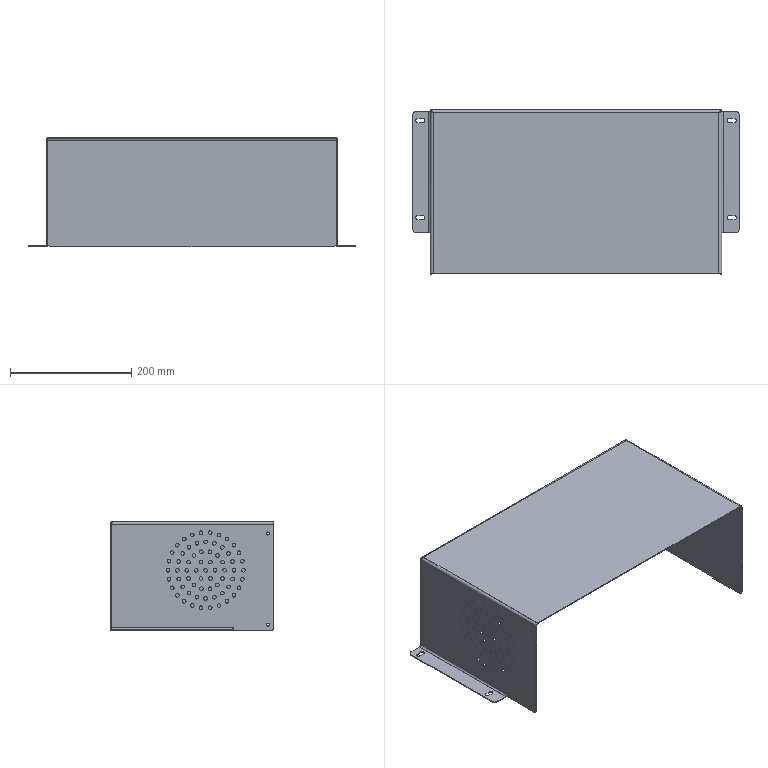Part | STEP file | 20-Motor cover | 1 solid | 228 faces | box 537 x 270 x 180 mm | volume 476658 mm3 | cylinder 172 | plane 52 | spline 4 | commonest cylinder face diameters 6 x139 7 x12 5 x8 10 x8 9 x5